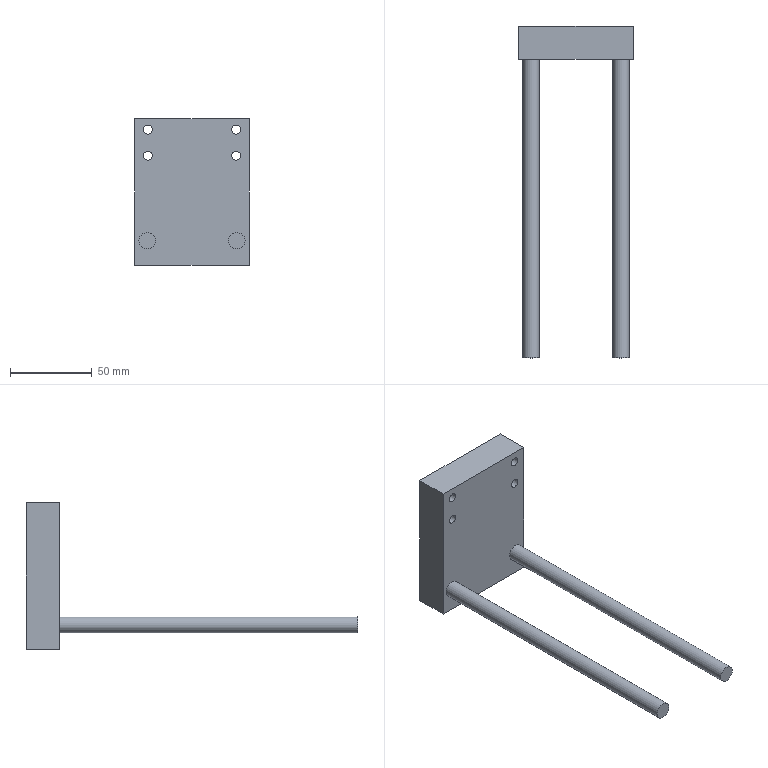Part | STEP file | Tube feed_id882_x_t | 1 solid | 30 faces | box 70 x 203.3 x 90 mm | volume 152546 mm3 | plane 16 | cylinder 14 | commonest cylinder face diameters 5.5 x6 8 x4 9 x2 10 x2